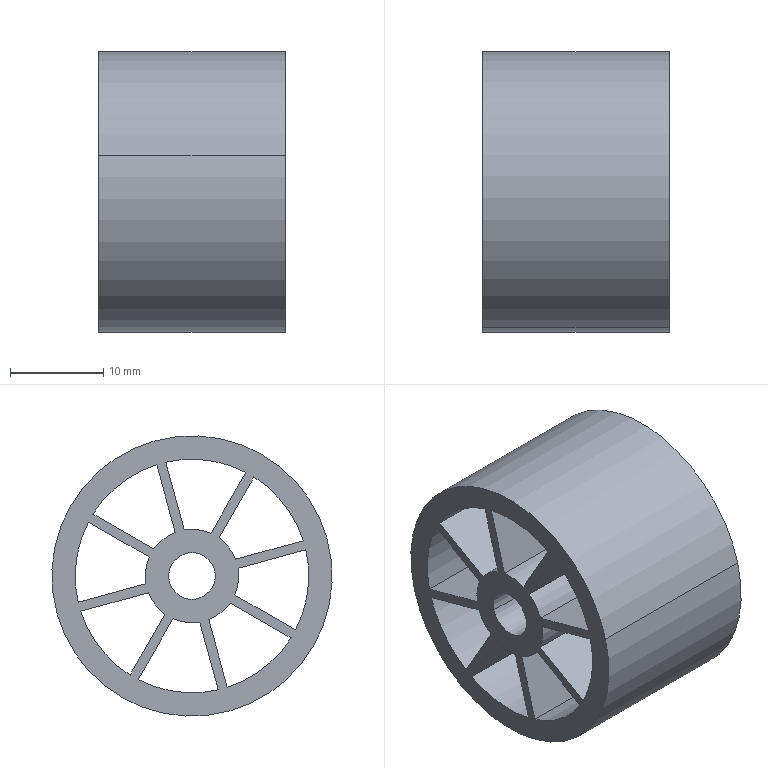Part | STEP file | Component42 | 1 solid | 38 faces | box 20 x 30 x 30 mm | volume 6699 mm3 | cylinder 20 | plane 18 | commonest cylinder face diameters 10 x8 25 x8 5 x2 30 x2
STEP:
#1=CARTESIAN_POINT('',(-10.,18.788,18.159));
#2=VERTEX_POINT('',#1);
#3=CARTESIAN_POINT('',(-10.,23.612,16.841));
#4=VERTEX_POINT('',#3);
#5=CARTESIAN_POINT('',(-10.,21.2,17.5));
#6=DIRECTION('',(1.,0.,0.));
#7=DIRECTION('',(0.,-0.9646,0.2636));
#8=AXIS2_PLACEMENT_3D('',#5,#6,#7);
#9=CIRCLE('',#8,2.5);
#10=EDGE_CURVE('',#2,#4,#9,.T.);
#11=ORIENTED_EDGE('',*,*,#10,.F.);
#12=CARTESIAN_POINT('',(10.,18.788,18.159));
#13=VERTEX_POINT('',#12);
#14=CARTESIAN_POINT('',(10.,18.788,18.159));
#15=DIRECTION('',(1.,0.,0.));
#16=VECTOR('',#15,1000.);
#17=LINE('',#14,#16);
#18=EDGE_CURVE('',#2,#13,#17,.T.);
#19=ORIENTED_EDGE('',*,*,#18,.T.);
#20=CARTESIAN_POINT('',(10.,23.612,16.841));
#21=VERTEX_POINT('',#20);
#22=CARTESIAN_POINT('',(10.,21.2,17.5));
#23=DIRECTION('',(1.,0.,0.));
#24=DIRECTION('',(0.,-0.9646,0.2636));
#25=AXIS2_PLACEMENT_3D('',#22,#23,#24);
#26=CIRCLE('',#25,2.5);
#27=EDGE_CURVE('',#13,#21,#26,.T.);
#28=ORIENTED_EDGE('',*,*,#27,.T.);
#29=CARTESIAN_POINT('',(10.,23.612,16.841));
#30=DIRECTION('',(1.,0.,0.));
#31=VECTOR('',#30,1000.);
#32=LINE('',#29,#31);
#33=EDGE_CURVE('',#4,#21,#32,.T.);
#34=ORIENTED_EDGE('',*,*,#33,.F.);
#35=EDGE_LOOP('',(#11,#19,#28,#34));
#36=FACE_OUTER_BOUND('',#35,.T.);
#37=CARTESIAN_POINT('',(10.,21.2,17.5));
#38=DIRECTION('',(1.,0.,0.));
#39=DIRECTION('',(0.,0.9646,-0.2636));
#40=AXIS2_PLACEMENT_3D('',#37,#38,#39);
#41=CYLINDRICAL_SURFACE('',#40,2.5);
#42=ADVANCED_FACE('',(#36),#41,.F.);
#43=CARTESIAN_POINT('',(-10.,35.67,13.547));
#44=VERTEX_POINT('',#43);
#45=CARTESIAN_POINT('',(-10.,6.73,21.453));
#46=VERTEX_POINT('',#45);
#47=CARTESIAN_POINT('',(-10.,21.2,17.5));
#48=DIRECTION('',(1.,0.,0.));
#49=DIRECTION('',(0.,-0.9646,0.2636));
#50=AXIS2_PLACEMENT_3D('',#47,#48,#49);
#51=CIRCLE('',#50,15.);
#52=EDGE_CURVE('',#44,#46,#51,.T.);
#53=ORIENTED_EDGE('',*,*,#52,.T.);
#54=CARTESIAN_POINT('',(10.,6.73,21.453));
#55=VERTEX_POINT('',#54);
#56=CARTESIAN_POINT('',(10.,6.73,21.453));
#57=DIRECTION('',(1.,0.,0.));
#58=VECTOR('',#57,1000.);
#59=LINE('',#56,#58);
#60=EDGE_CURVE('',#46,#55,#59,.T.);
#61=ORIENTED_EDGE('',*,*,#60,.T.);
#62=CARTESIAN_POINT('',(10.,35.67,13.547));
#63=VERTEX_POINT('',#62);
#64=CARTESIAN_POINT('',(10.,21.2,17.5));
#65=DIRECTION('',(1.,0.,0.));
#66=DIRECTION('',(0.,-0.9646,0.2636));
#67=AXIS2_PLACEMENT_3D('',#64,#65,#66);
#68=CIRCLE('',#67,15.);
#69=EDGE_CURVE('',#63,#55,#68,.T.);
#70=ORIENTED_EDGE('',*,*,#69,.F.);
#71=CARTESIAN_POINT('',(10.,35.67,13.547));
#72=DIRECTION('',(1.,0.,0.));
#73=VECTOR('',#72,1000.);
#74=LINE('',#71,#73);
#75=EDGE_CURVE('',#44,#63,#74,.T.);
#76=ORIENTED_EDGE('',*,*,#75,.F.);
#77=EDGE_LOOP('',(#53,#61,#70,#76));
#78=FACE_OUTER_BOUND('',#77,.T.);
#79=CARTESIAN_POINT('',(10.,21.2,17.5));
#80=DIRECTION('',(1.,0.,0.));
#81=DIRECTION('',(0.,0.9646,-0.2636));
#82=AXIS2_PLACEMENT_3D('',#79,#80,#81);
#83=CYLINDRICAL_SURFACE('',#82,15.);
#84=ADVANCED_FACE('',(#78),#83,.T.);
#85=CARTESIAN_POINT('',(10.,33.117,13.726));
#86=VERTEX_POINT('',#85);
#87=CARTESIAN_POINT('',(10.,25.867,15.706));
#88=VERTEX_POINT('',#87);
#89=CARTESIAN_POINT('',(10.,33.117,13.726));
#90=DIRECTION('',(0.,-0.9646,0.2636));
#91=VECTOR('',#90,1000.);
#92=LINE('',#89,#91);
#93=EDGE_CURVE('',#86,#88,#92,.T.);
#94=ORIENTED_EDGE('',*,*,#93,.T.);
#95=CARTESIAN_POINT('',(-10.,25.867,15.706));
#96=VERTEX_POINT('',#95);
#97=CARTESIAN_POINT('',(-10.,25.867,15.706));
#98=DIRECTION('',(1.,0.,0.));
#99=VECTOR('',#98,1000.);
#100=LINE('',#97,#99);
#101=EDGE_CURVE('',#96,#88,#100,.T.);
#102=ORIENTED_EDGE('',*,*,#101,.F.);
#103=CARTESIAN_POINT('',(-10.,33.117,13.726));
#104=VERTEX_POINT('',#103);
#105=CARTESIAN_POINT('',(-10.,33.117,13.726));
#106=DIRECTION('',(0.,-0.9646,0.2636));
#107=VECTOR('',#106,1000.);
#108=LINE('',#105,#107);
#109=EDGE_CURVE('',#104,#96,#108,.T.);
#110=ORIENTED_EDGE('',*,*,#109,.F.);
#111=CARTESIAN_POINT('',(-10.,33.117,13.726));
#112=DIRECTION('',(1.,0.,0.));
#113=VECTOR('',#112,1000.);
#114=LINE('',#111,#113);
#115=EDGE_CURVE('',#104,#86,#114,.T.);
#116=ORIENTED_EDGE('',*,*,#115,.T.);
#117=EDGE_LOOP('',(#94,#102,#110,#116));
#118=FACE_OUTER_BOUND('',#117,.T.);
#119=CARTESIAN_POINT('',(-10.,29.492,14.716));
#120=DIRECTION('',(0.,0.2636,0.9646));
#121=DIRECTION('',(1.,0.,0.));
#122=AXIS2_PLACEMENT_3D('',#119,#120,#121);
#123=PLANE('',#122);
#124=ADVANCED_FACE('',(#118),#123,.F.);
#125=CARTESIAN_POINT('',(10.,27.826,6.901));
#126=VERTEX_POINT('',#125);
#127=CARTESIAN_POINT('',(10.,21.2,17.5));
#128=DIRECTION('',(1.,0.,0.));
#129=DIRECTION('',(0.,-0.9646,0.2636));
#130=AXIS2_PLACEMENT_3D('',#127,#128,#129);
#131=CIRCLE('',#130,12.5);
#132=EDGE_CURVE('',#126,#86,#131,.T.);
#133=ORIENTED_EDGE('',*,*,#132,.T.);
#134=ORIENTED_EDGE('',*,*,#115,.F.);
#135=CARTESIAN_POINT('',(-10.,27.826,6.901));
#136=VERTEX_POINT('',#135);
#137=CARTESIAN_POINT('',(-10.,21.2,17.5));
#138=DIRECTION('',(1.,0.,0.));
#139=DIRECTION('',(0.,-0.9646,0.2636));
#140=AXIS2_PLACEMENT_3D('',#137,#138,#139);
#141=CIRCLE('',#140,12.5);
#142=EDGE_CURVE('',#136,#104,#141,.T.);
#143=ORIENTED_EDGE('',*,*,#142,.F.);
#144=CARTESIAN_POINT('',(-10.,27.826,6.901));
#145=DIRECTION('',(1.,0.,0.));
#146=VECTOR('',#145,1000.);
#147=LINE('',#144,#146);
#148=EDGE_CURVE('',#136,#126,#147,.T.);
#149=ORIENTED_EDGE('',*,*,#148,.T.);
#150=EDGE_LOOP('',(#133,#134,#143,#149));
#151=FACE_OUTER_BOUND('',#150,.T.);
#152=CARTESIAN_POINT('',(-10.,21.2,17.5));
#153=DIRECTION('',(-1.,0.,0.));
#154=DIRECTION('',(0.,-0.9646,0.2636));
#155=AXIS2_PLACEMENT_3D('',#152,#153,#154);
#156=CYLINDRICAL_SURFACE('',#155,12.5);
#157=ADVANCED_FACE('',(#151),#156,.F.);
#158=CARTESIAN_POINT('',(10.,24.101,13.427));
#159=VERTEX_POINT('',#158);
#160=CARTESIAN_POINT('',(10.,24.101,13.427));
#161=DIRECTION('',(0.,0.4957,-0.8685));
#162=VECTOR('',#161,1000.);
#163=LINE('',#160,#162);
#164=EDGE_CURVE('',#159,#126,#163,.T.);
#165=ORIENTED_EDGE('',*,*,#164,.T.);
#166=ORIENTED_EDGE('',*,*,#148,.F.);
#167=CARTESIAN_POINT('',(-10.,24.101,13.427));
#168=VERTEX_POINT('',#167);
#169=CARTESIAN_POINT('',(-10.,24.101,13.427));
#170=DIRECTION('',(0.,0.4957,-0.8685));
#171=VECTOR('',#170,1000.);
#172=LINE('',#169,#171);
#173=EDGE_CURVE('',#168,#136,#172,.T.);
#174=ORIENTED_EDGE('',*,*,#173,.F.);
#175=CARTESIAN_POINT('',(-10.,24.101,13.427));
#176=DIRECTION('',(1.,0.,0.));
#177=VECTOR('',#176,1000.);
#178=LINE('',#175,#177);
#179=EDGE_CURVE('',#168,#159,#178,.T.);
#180=ORIENTED_EDGE('',*,*,#179,.T.);
#181=EDGE_LOOP('',(#165,#166,#174,#180));
#182=FACE_OUTER_BOUND('',#181,.T.);
#183=CARTESIAN_POINT('',(-10.,25.963,10.164));
#184=DIRECTION('',(0.,-0.8685,-0.4957));
#185=DIRECTION('',(0.,0.4957,-0.8685));
#186=AXIS2_PLACEMENT_3D('',#183,#184,#185);
#187=PLANE('',#186);
#188=ADVANCED_FACE('',(#182),#187,.F.);
#189=CARTESIAN_POINT('',(10.,21.2,17.5));
#190=DIRECTION('',(-1.,0.,0.));
#191=DIRECTION('',(0.,-0.9646,0.2636));
#192=AXIS2_PLACEMENT_3D('',#189,#190,#191);
#193=CIRCLE('',#192,5.);
#194=EDGE_CURVE('',#88,#159,#193,.T.);
#195=ORIENTED_EDGE('',*,*,#194,.T.);
#196=ORIENTED_EDGE('',*,*,#179,.F.);
#197=CARTESIAN_POINT('',(-10.,21.2,17.5));
#198=DIRECTION('',(-1.,0.,0.));
#199=DIRECTION('',(0.,-0.9646,0.2636));
#200=AXIS2_PLACEMENT_3D('',#197,#198,#199);
#201=CIRCLE('',#200,5.);
#202=EDGE_CURVE('',#96,#168,#201,.T.);
#203=ORIENTED_EDGE('',*,*,#202,.F.);
#204=ORIENTED_EDGE('',*,*,#101,.T.);
#205=EDGE_LOOP('',(#195,#196,#203,#204));
#206=FACE_OUTER_BOUND('',#205,.T.);
#207=CARTESIAN_POINT('',(-10.,21.2,17.5));
#208=DIRECTION('',(-1.,0.,0.));
#209=DIRECTION('',(0.,-0.9646,0.2636));
#210=AXIS2_PLACEMENT_3D('',#207,#208,#209);
#211=CYLINDRICAL_SURFACE('',#210,5.);
#212=ADVANCED_FACE('',(#206),#211,.T.);
#213=CARTESIAN_POINT('',(10.,32.295,23.258));
#214=VERTEX_POINT('',#213);
#215=CARTESIAN_POINT('',(10.,25.768,19.532));
#216=VERTEX_POINT('',#215);
#217=CARTESIAN_POINT('',(10.,32.295,23.258));
#218=DIRECTION('',(0.,-0.8685,-0.4957));
#219=VECTOR('',#218,1000.);
#220=LINE('',#217,#219);
#221=EDGE_CURVE('',#214,#216,#220,.T.);
#222=ORIENTED_EDGE('',*,*,#221,.T.);
#223=CARTESIAN_POINT('',(-10.,25.768,19.532));
#224=VERTEX_POINT('',#223);
#225=CARTESIAN_POINT('',(-10.,25.768,19.532));
#226=DIRECTION('',(1.,0.,0.));
#227=VECTOR('',#226,1000.);
#228=LINE('',#225,#227);
#229=EDGE_CURVE('',#224,#216,#228,.T.);
#230=ORIENTED_EDGE('',*,*,#229,.F.);
#231=CARTESIAN_POINT('',(-10.,32.295,23.258));
#232=VERTEX_POINT('',#231);
#233=CARTESIAN_POINT('',(-10.,32.295,23.258));
#234=DIRECTION('',(0.,-0.8685,-0.4957));
#235=VECTOR('',#234,1000.);
#236=LINE('',#233,#235);
#237=EDGE_CURVE('',#232,#224,#236,.T.);
#238=ORIENTED_EDGE('',*,*,#237,.F.);
#239=CARTESIAN_POINT('',(-10.,32.295,23.258));
#240=DIRECTION('',(1.,0.,0.));
#241=VECTOR('',#240,1000.);
#242=LINE('',#239,#241);
#243=EDGE_CURVE('',#232,#214,#242,.T.);
#244=ORIENTED_EDGE('',*,*,#243,.T.);
#245=EDGE_LOOP('',(#222,#230,#238,#244));
#246=FACE_OUTER_BOUND('',#245,.T.);
#247=CARTESIAN_POINT('',(-10.,29.032,21.395));
#248=DIRECTION('',(0.,-0.4957,0.8685));
#249=DIRECTION('',(-1.,0.,0.));
#250=AXIS2_PLACEMENT_3D('',#247,#248,#249);
#251=PLANE('',#250);
#252=ADVANCED_FACE('',(#246),#251,.F.);
#253=CARTESIAN_POINT('',(10.,33.38,14.69));
#254=VERTEX_POINT('',#253);
#255=CARTESIAN_POINT('',(10.,21.2,17.5));
#256=DIRECTION('',(1.,0.,0.));
#257=DIRECTION('',(0.,-0.9646,0.2636));
#258=AXIS2_PLACEMENT_3D('',#255,#256,#257);
#259=CIRCLE('',#258,12.5);
#260=EDGE_CURVE('',#254,#214,#259,.T.);
#261=ORIENTED_EDGE('',*,*,#260,.T.);
#262=ORIENTED_EDGE('',*,*,#243,.F.);
#263=CARTESIAN_POINT('',(-10.,33.38,14.69));
#264=VERTEX_POINT('',#263);
#265=CARTESIAN_POINT('',(-10.,21.2,17.5));
#266=DIRECTION('',(1.,0.,0.));
#267=DIRECTION('',(0.,-0.9646,0.2636));
#268=AXIS2_PLACEMENT_3D('',#265,#266,#267);
#269=CIRCLE('',#268,12.5);
#270=EDGE_CURVE('',#264,#232,#269,.T.);
#271=ORIENTED_EDGE('',*,*,#270,.F.);
#272=CARTESIAN_POINT('',(-10.,33.38,14.69));
#273=DIRECTION('',(1.,0.,0.));
#274=VECTOR('',#273,1000.);
#275=LINE('',#272,#274);
#276=EDGE_CURVE('',#264,#254,#275,.T.);
#277=ORIENTED_EDGE('',*,*,#276,.T.);
#278=EDGE_LOOP('',(#261,#262,#271,#277));
#279=FACE_OUTER_BOUND('',#278,.T.);
#280=CARTESIAN_POINT('',(-10.,21.2,17.5));
#281=DIRECTION('',(-1.,0.,0.));
#282=DIRECTION('',(0.,-0.9646,0.2636));
#283=AXIS2_PLACEMENT_3D('',#280,#281,#282);
#284=CYLINDRICAL_SURFACE('',#283,12.5);
#285=ADVANCED_FACE('',(#279),#284,.F.);
#286=CARTESIAN_POINT('',(10.,26.131,16.671));
#287=VERTEX_POINT('',#286);
#288=CARTESIAN_POINT('',(10.,26.131,16.671));
#289=DIRECTION('',(0.,0.9646,-0.2636));
#290=VECTOR('',#289,1000.);
#291=LINE('',#288,#290);
#292=EDGE_CURVE('',#287,#254,#291,.T.);
#293=ORIENTED_EDGE('',*,*,#292,.T.);
#294=ORIENTED_EDGE('',*,*,#276,.F.);
#295=CARTESIAN_POINT('',(-10.,26.131,16.671));
#296=VERTEX_POINT('',#295);
#297=CARTESIAN_POINT('',(-10.,26.131,16.671));
#298=DIRECTION('',(0.,0.9646,-0.2636));
#299=VECTOR('',#298,1000.);
#300=LINE('',#297,#299);
#301=EDGE_CURVE('',#296,#264,#300,.T.);
#302=ORIENTED_EDGE('',*,*,#301,.F.);
#303=CARTESIAN_POINT('',(-10.,26.131,16.671));
#304=DIRECTION('',(1.,0.,0.));
#305=VECTOR('',#304,1000.);
#306=LINE('',#303,#305);
#307=EDGE_CURVE('',#296,#287,#306,.T.);
#308=ORIENTED_EDGE('',*,*,#307,.T.);
#309=EDGE_LOOP('',(#293,#294,#302,#308));
#310=FACE_OUTER_BOUND('',#309,.T.);
#311=CARTESIAN_POINT('',(-10.,29.755,15.681));
#312=DIRECTION('',(0.,-0.2636,-0.9646));
#313=DIRECTION('',(0.,-0.9646,0.2636));
#314=AXIS2_PLACEMENT_3D('',#311,#312,#313);
#315=PLANE('',#314);
#316=ADVANCED_FACE('',(#310),#315,.F.);
#317=CARTESIAN_POINT('',(10.,21.2,17.5));
#318=DIRECTION('',(-1.,0.,0.));
#319=DIRECTION('',(0.,-0.9646,0.2636));
#320=AXIS2_PLACEMENT_3D('',#317,#318,#319);
#321=CIRCLE('',#320,5.);
#322=EDGE_CURVE('',#216,#287,#321,.T.);
#323=ORIENTED_EDGE('',*,*,#322,.T.);
#324=ORIENTED_EDGE('',*,*,#307,.F.);
#325=CARTESIAN_POINT('',(-10.,21.2,17.5));
#326=DIRECTION('',(-1.,0.,0.));
#327=DIRECTION('',(0.,-0.9646,0.2636));
#328=AXIS2_PLACEMENT_3D('',#325,#326,#327);
#329=CIRCLE('',#328,5.);
#330=EDGE_CURVE('',#224,#296,#329,.T.);
#331=ORIENTED_EDGE('',*,*,#330,.F.);
#332=ORIENTED_EDGE('',*,*,#229,.T.);
#333=EDGE_LOOP('',(#323,#324,#331,#332));
#334=FACE_OUTER_BOUND('',#333,.T.);
#335=CARTESIAN_POINT('',(-10.,21.2,17.5));
#336=DIRECTION('',(-1.,0.,0.));
#337=DIRECTION('',(0.,-0.9646,0.2636));
#338=AXIS2_PLACEMENT_3D('',#335,#336,#337);
#339=CYLINDRICAL_SURFACE('',#338,5.);
#340=ADVANCED_FACE('',(#334),#339,.T.);
#341=CARTESIAN_POINT('',(10.,24.974,29.417));
#342=VERTEX_POINT('',#341);
#343=CARTESIAN_POINT('',(10.,22.994,22.167));
#344=VERTEX_POINT('',#343);
#345=CARTESIAN_POINT('',(10.,24.974,29.417));
#346=DIRECTION('',(0.,-0.2636,-0.9646));
#347=VECTOR('',#346,1000.);
#348=LINE('',#345,#347);
#349=EDGE_CURVE('',#342,#344,#348,.T.);
#350=ORIENTED_EDGE('',*,*,#349,.T.);
#351=CARTESIAN_POINT('',(-10.,22.994,22.167));
#352=VERTEX_POINT('',#351);
#353=CARTESIAN_POINT('',(-10.,22.994,22.167));
#354=DIRECTION('',(1.,0.,0.));
#355=VECTOR('',#354,1000.);
#356=LINE('',#353,#355);
#357=EDGE_CURVE('',#352,#344,#356,.T.);
#358=ORIENTED_EDGE('',*,*,#357,.F.);
#359=CARTESIAN_POINT('',(-10.,24.974,29.417));
#360=VERTEX_POINT('',#359);
#361=CARTESIAN_POINT('',(-10.,24.974,29.417));
#362=DIRECTION('',(0.,-0.2636,-0.9646));
#363=VECTOR('',#362,1000.);
#364=LINE('',#361,#363);
#365=EDGE_CURVE('',#360,#352,#364,.T.);
#366=ORIENTED_EDGE('',*,*,#365,.F.);
#367=CARTESIAN_POINT('',(-10.,24.974,29.417));
#368=DIRECTION('',(1.,0.,0.));
#369=VECTOR('',#368,1000.);
#370=LINE('',#367,#369);
#371=EDGE_CURVE('',#360,#342,#370,.T.);
#372=ORIENTED_EDGE('',*,*,#371,.T.);
#373=EDGE_LOOP('',(#350,#358,#366,#372));
#374=FACE_OUTER_BOUND('',#373,.T.);
#375=CARTESIAN_POINT('',(-10.,23.984,25.792));
#376=DIRECTION('',(0.,-0.9646,0.2636));
#377=DIRECTION('',(-1.,0.,0.));
#378=AXIS2_PLACEMENT_3D('',#375,#376,#377);
#379=PLANE('',#378);
#380=ADVANCED_FACE('',(#374),#379,.F.);
#381=CARTESIAN_POINT('',(10.,31.799,24.126));
#382=VERTEX_POINT('',#381);
#383=CARTESIAN_POINT('',(10.,21.2,17.5));
#384=DIRECTION('',(1.,0.,0.));
#385=DIRECTION('',(0.,-0.9646,0.2636));
#386=AXIS2_PLACEMENT_3D('',#383,#384,#385);
#387=CIRCLE('',#386,12.5);
#388=EDGE_CURVE('',#382,#342,#387,.T.);
#389=ORIENTED_EDGE('',*,*,#388,.T.);
#390=ORIENTED_EDGE('',*,*,#371,.F.);
#391=CARTESIAN_POINT('',(-10.,31.799,24.126));
#392=VERTEX_POINT('',#391);
#393=CARTESIAN_POINT('',(-10.,21.2,17.5));
#394=DIRECTION('',(1.,0.,0.));
#395=DIRECTION('',(0.,-0.9646,0.2636));
#396=AXIS2_PLACEMENT_3D('',#393,#394,#395);
#397=CIRCLE('',#396,12.5);
#398=EDGE_CURVE('',#392,#360,#397,.T.);
#399=ORIENTED_EDGE('',*,*,#398,.F.);
#400=CARTESIAN_POINT('',(-10.,31.799,24.126));
#401=DIRECTION('',(1.,0.,0.));
#402=VECTOR('',#401,1000.);
#403=LINE('',#400,#402);
#404=EDGE_CURVE('',#392,#382,#403,.T.);
#405=ORIENTED_EDGE('',*,*,#404,.T.);
#406=EDGE_LOOP('',(#389,#390,#399,#405));
#407=FACE_OUTER_BOUND('',#406,.T.);
#408=CARTESIAN_POINT('',(-10.,21.2,17.5));
#409=DIRECTION('',(-1.,0.,0.));
#410=DIRECTION('',(0.,-0.9646,0.2636));
#411=AXIS2_PLACEMENT_3D('',#408,#409,#410);
#412=CYLINDRICAL_SURFACE('',#411,12.5);
#413=ADVANCED_FACE('',(#407),#412,.F.);
#414=CARTESIAN_POINT('',(10.,25.273,20.401));
#415=VERTEX_POINT('',#414);
#416=CARTESIAN_POINT('',(10.,25.273,20.401));
#417=DIRECTION('',(0.,0.8685,0.4957));
#418=VECTOR('',#417,1000.);
#419=LINE('',#416,#418);
#420=EDGE_CURVE('',#415,#382,#419,.T.);
#421=ORIENTED_EDGE('',*,*,#420,.T.);
#422=ORIENTED_EDGE('',*,*,#404,.F.);
#423=CARTESIAN_POINT('',(-10.,25.273,20.401));
#424=VERTEX_POINT('',#423);
#425=CARTESIAN_POINT('',(-10.,25.273,20.401));
#426=DIRECTION('',(0.,0.8685,0.4957));
#427=VECTOR('',#426,1000.);
#428=LINE('',#425,#427);
#429=EDGE_CURVE('',#424,#392,#428,.T.);
#430=ORIENTED_EDGE('',*,*,#429,.F.);
#431=CARTESIAN_POINT('',(-10.,25.273,20.401));
#432=DIRECTION('',(1.,0.,0.));
#433=VECTOR('',#432,1000.);
#434=LINE('',#431,#433);
#435=EDGE_CURVE('',#424,#415,#434,.T.);
#436=ORIENTED_EDGE('',*,*,#435,.T.);
#437=EDGE_LOOP('',(#421,#422,#430,#436));
#438=FACE_OUTER_BOUND('',#437,.T.);
#439=CARTESIAN_POINT('',(-10.,28.536,22.263));
#440=DIRECTION('',(0.,0.4957,-0.8685));
#441=DIRECTION('',(-1.,0.,0.));
#442=AXIS2_PLACEMENT_3D('',#439,#440,#441);
#443=PLANE('',#442);
#444=ADVANCED_FACE('',(#438),#443,.F.);
#445=CARTESIAN_POINT('',(10.,21.2,17.5));
#446=DIRECTION('',(-1.,0.,0.));
#447=DIRECTION('',(0.,-0.9646,0.2636));
#448=AXIS2_PLACEMENT_3D('',#445,#446,#447);
#449=CIRCLE('',#448,5.);
#450=EDGE_CURVE('',#344,#415,#449,.T.);
#451=ORIENTED_EDGE('',*,*,#450,.T.);
#452=ORIENTED_EDGE('',*,*,#435,.F.);
#453=CARTESIAN_POINT('',(-10.,21.2,17.5));
#454=DIRECTION('',(-1.,0.,0.));
#455=DIRECTION('',(0.,-0.9646,0.2636));
#456=AXIS2_PLACEMENT_3D('',#453,#454,#455);
#457=CIRCLE('',#456,5.);
#458=EDGE_CURVE('',#352,#424,#457,.T.);
#459=ORIENTED_EDGE('',*,*,#458,.F.);
#460=ORIENTED_EDGE('',*,*,#357,.T.);
#461=EDGE_LOOP('',(#451,#452,#459,#460));
#462=FACE_OUTER_BOUND('',#461,.T.);
#463=CARTESIAN_POINT('',(-10.,21.2,17.5));
#464=DIRECTION('',(-1.,0.,0.));
#465=DIRECTION('',(0.,-0.9646,0.2636));
#466=AXIS2_PLACEMENT_3D('',#463,#464,#465);
#467=CYLINDRICAL_SURFACE('',#466,5.);
#468=ADVANCED_FACE('',(#462),#467,.T.);
#469=CARTESIAN_POINT('',(10.,15.442,28.595));
#470=VERTEX_POINT('',#469);
#471=CARTESIAN_POINT('',(10.,19.168,22.068));
#472=VERTEX_POINT('',#471);
#473=CARTESIAN_POINT('',(10.,15.442,28.595));
#474=DIRECTION('',(0.,0.4957,-0.8685));
#475=VECTOR('',#474,1000.);
#476=LINE('',#473,#475);
#477=EDGE_CURVE('',#470,#472,#476,.T.);
#478=ORIENTED_EDGE('',*,*,#477,.T.);
#479=CARTESIAN_POINT('',(-10.,19.168,22.068));
#480=VERTEX_POINT('',#479);
#481=CARTESIAN_POINT('',(-10.,19.168,22.068));
#482=DIRECTION('',(1.,0.,0.));
#483=VECTOR('',#482,1000.);
#484=LINE('',#481,#483);
#485=EDGE_CURVE('',#480,#472,#484,.T.);
#486=ORIENTED_EDGE('',*,*,#485,.F.);
#487=CARTESIAN_POINT('',(-10.,15.442,28.595));
#488=VERTEX_POINT('',#487);
#489=CARTESIAN_POINT('',(-10.,15.442,28.595));
#490=DIRECTION('',(0.,0.4957,-0.8685));
#491=VECTOR('',#490,1000.);
#492=LINE('',#489,#491);
#493=EDGE_CURVE('',#488,#480,#492,.T.);
#494=ORIENTED_EDGE('',*,*,#493,.F.);
#495=CARTESIAN_POINT('',(-10.,15.442,28.595));
#496=DIRECTION('',(1.,0.,0.));
#497=VECTOR('',#496,1000.);
#498=LINE('',#495,#497);
#499=EDGE_CURVE('',#488,#470,#498,.T.);
#500=ORIENTED_EDGE('',*,*,#499,.T.);
#501=EDGE_LOOP('',(#478,#486,#494,#500));
#502=FACE_OUTER_BOUND('',#501,.T.);
#503=CARTESIAN_POINT('',(-10.,17.305,25.332));
#504=DIRECTION('',(0.,-0.8685,-0.4957));
#505=DIRECTION('',(0.,0.4957,-0.8685));
#506=AXIS2_PLACEMENT_3D('',#503,#504,#505);
#507=PLANE('',#506);
#508=ADVANCED_FACE('',(#502),#507,.F.);
#509=CARTESIAN_POINT('',(10.,24.01,29.68));
#510=VERTEX_POINT('',#509);
#511=CARTESIAN_POINT('',(10.,21.2,17.5));
#512=DIRECTION('',(1.,0.,0.));
#513=DIRECTION('',(0.,-0.9646,0.2636));
#514=AXIS2_PLACEMENT_3D('',#511,#512,#513);
#515=CIRCLE('',#514,12.5);
#516=EDGE_CURVE('',#510,#470,#515,.T.);
#517=ORIENTED_EDGE('',*,*,#516,.T.);
#518=ORIENTED_EDGE('',*,*,#499,.F.);
#519=CARTESIAN_POINT('',(-10.,24.01,29.68));
#520=VERTEX_POINT('',#519);
#521=CARTESIAN_POINT('',(-10.,21.2,17.5));
#522=DIRECTION('',(1.,0.,0.));
#523=DIRECTION('',(0.,-0.9646,0.2636));
#524=AXIS2_PLACEMENT_3D('',#521,#522,#523);
#525=CIRCLE('',#524,12.5);
#526=EDGE_CURVE('',#520,#488,#525,.T.);
#527=ORIENTED_EDGE('',*,*,#526,.F.);
#528=CARTESIAN_POINT('',(-10.,24.01,29.68));
#529=DIRECTION('',(1.,0.,0.));
#530=VECTOR('',#529,1000.);
#531=LINE('',#528,#530);
#532=EDGE_CURVE('',#520,#510,#531,.T.);
#533=ORIENTED_EDGE('',*,*,#532,.T.);
#534=EDGE_LOOP('',(#517,#518,#527,#533));
#535=FACE_OUTER_BOUND('',#534,.T.);
#536=CARTESIAN_POINT('',(-10.,21.2,17.5));
#537=DIRECTION('',(-1.,0.,0.));
#538=DIRECTION('',(0.,-0.9646,0.2636));
#539=AXIS2_PLACEMENT_3D('',#536,#537,#538);
#540=CYLINDRICAL_SURFACE('',#539,12.5);
#541=ADVANCED_FACE('',(#535),#540,.F.);
#542=CARTESIAN_POINT('',(10.,22.029,22.431));
#543=VERTEX_POINT('',#542);
#544=CARTESIAN_POINT('',(10.,22.029,22.431));
#545=DIRECTION('',(0.,0.2636,0.9646));
#546=VECTOR('',#545,1000.);
#547=LINE('',#544,#546);
#548=EDGE_CURVE('',#543,#510,#547,.T.);
#549=ORIENTED_EDGE('',*,*,#548,.T.);
#550=ORIENTED_EDGE('',*,*,#532,.F.);
#551=CARTESIAN_POINT('',(-10.,22.029,22.431));
#552=VERTEX_POINT('',#551);
#553=CARTESIAN_POINT('',(-10.,22.029,22.431));
#554=DIRECTION('',(0.,0.2636,0.9646));
#555=VECTOR('',#554,1000.);
#556=LINE('',#553,#555);
#557=EDGE_CURVE('',#552,#520,#556,.T.);
#558=ORIENTED_EDGE('',*,*,#557,.F.);
#559=CARTESIAN_POINT('',(-10.,22.029,22.431));
#560=DIRECTION('',(1.,0.,0.));
#561=VECTOR('',#560,1000.);
#562=LINE('',#559,#561);
#563=EDGE_CURVE('',#552,#543,#562,.T.);
#564=ORIENTED_EDGE('',*,*,#563,.T.);
#565=EDGE_LOOP('',(#549,#550,#558,#564));
#566=FACE_OUTER_BOUND('',#565,.T.);
#567=CARTESIAN_POINT('',(-10.,23.019,26.055));
#568=DIRECTION('',(0.,0.9646,-0.2636));
#569=DIRECTION('',(-1.,0.,0.));
#570=AXIS2_PLACEMENT_3D('',#567,#568,#569);
#571=PLANE('',#570);
#572=ADVANCED_FACE('',(#566),#571,.F.);
#573=CARTESIAN_POINT('',(10.,21.2,17.5));
#574=DIRECTION('',(-1.,0.,0.));
#575=DIRECTION('',(0.,-0.9646,0.2636));
#576=AXIS2_PLACEMENT_3D('',#573,#574,#575);
#577=CIRCLE('',#576,5.);
#578=EDGE_CURVE('',#472,#543,#577,.T.);
#579=ORIENTED_EDGE('',*,*,#578,.T.);
#580=ORIENTED_EDGE('',*,*,#563,.F.);
#581=CARTESIAN_POINT('',(-10.,21.2,17.5));
#582=DIRECTION('',(-1.,0.,0.));
#583=DIRECTION('',(0.,-0.9646,0.2636));
#584=AXIS2_PLACEMENT_3D('',#581,#582,#583);
#585=CIRCLE('',#584,5.);
#586=EDGE_CURVE('',#480,#552,#585,.T.);
#587=ORIENTED_EDGE('',*,*,#586,.F.);
#588=ORIENTED_EDGE('',*,*,#485,.T.);
#589=EDGE_LOOP('',(#579,#580,#587,#588));
#590=FACE_OUTER_BOUND('',#589,.T.);
#591=CARTESIAN_POINT('',(-10.,21.2,17.5));
#592=DIRECTION('',(-1.,0.,0.));
#593=DIRECTION('',(0.,-0.9646,0.2636));
#594=AXIS2_PLACEMENT_3D('',#591,#592,#593);
#595=CYLINDRICAL_SURFACE('',#594,5.);
#596=ADVANCED_FACE('',(#590),#595,.T.);
#597=CARTESIAN_POINT('',(10.,9.283,21.274));
#598=VERTEX_POINT('',#597);
#599=CARTESIAN_POINT('',(10.,16.533,19.294));
#600=VERTEX_POINT('',#599);
#601=CARTESIAN_POINT('',(10.,9.283,21.274));
#602=DIRECTION('',(0.,0.9646,-0.2636));
#603=VECTOR('',#602,1000.);
#604=LINE('',#601,#603);
#605=EDGE_CURVE('',#598,#600,#604,.T.);
#606=ORIENTED_EDGE('',*,*,#605,.T.);
#607=CARTESIAN_POINT('',(-10.,16.533,19.294));
#608=VERTEX_POINT('',#607);
#609=CARTESIAN_POINT('',(-10.,16.533,19.294));
#610=DIRECTION('',(1.,0.,0.));
#611=VECTOR('',#610,1000.);
#612=LINE('',#609,#611);
#613=EDGE_CURVE('',#608,#600,#612,.T.);
#614=ORIENTED_EDGE('',*,*,#613,.F.);
#615=CARTESIAN_POINT('',(-10.,9.283,21.274));
#616=VERTEX_POINT('',#615);
#617=CARTESIAN_POINT('',(-10.,9.283,21.274));
#618=DIRECTION('',(0.,0.9646,-0.2636));
#619=VECTOR('',#618,1000.);
#620=LINE('',#617,#619);
#621=EDGE_CURVE('',#616,#608,#620,.T.);
#622=ORIENTED_EDGE('',*,*,#621,.F.);
#623=CARTESIAN_POINT('',(-10.,9.283,21.274));
#624=DIRECTION('',(1.,0.,0.));
#625=VECTOR('',#624,1000.);
#626=LINE('',#623,#625);
#627=EDGE_CURVE('',#616,#598,#626,.T.);
#628=ORIENTED_EDGE('',*,*,#627,.T.);
#629=EDGE_LOOP('',(#606,#614,#622,#628));
#630=FACE_OUTER_BOUND('',#629,.T.);
#631=CARTESIAN_POINT('',(-10.,12.908,20.284));
#632=DIRECTION('',(0.,-0.2636,-0.9646));
#633=DIRECTION('',(0.,-0.9646,0.2636));
#634=AXIS2_PLACEMENT_3D('',#631,#632,#633);
#635=PLANE('',#634);
#636=ADVANCED_FACE('',(#630),#635,.F.);
#637=CARTESIAN_POINT('',(10.,14.574,28.099));
#638=VERTEX_POINT('',#637);
#639=CARTESIAN_POINT('',(10.,21.2,17.5));
#640=DIRECTION('',(1.,0.,0.));
#641=DIRECTION('',(0.,-0.9646,0.2636));
#642=AXIS2_PLACEMENT_3D('',#639,#640,#641);
#643=CIRCLE('',#642,12.5);
#644=EDGE_CURVE('',#638,#598,#643,.T.);
#645=ORIENTED_EDGE('',*,*,#644,.T.);
#646=ORIENTED_EDGE('',*,*,#627,.F.);
#647=CARTESIAN_POINT('',(-10.,14.574,28.099));
#648=VERTEX_POINT('',#647);
#649=CARTESIAN_POINT('',(-10.,21.2,17.5));
#650=DIRECTION('',(1.,0.,0.));
#651=DIRECTION('',(0.,-0.9646,0.2636));
#652=AXIS2_PLACEMENT_3D('',#649,#650,#651);
#653=CIRCLE('',#652,12.5);
#654=EDGE_CURVE('',#648,#616,#653,.T.);
#655=ORIENTED_EDGE('',*,*,#654,.F.);
#656=CARTESIAN_POINT('',(-10.,14.574,28.099));
#657=DIRECTION('',(1.,0.,0.));
#658=VECTOR('',#657,1000.);
#659=LINE('',#656,#658);
#660=EDGE_CURVE('',#648,#638,#659,.T.);
#661=ORIENTED_EDGE('',*,*,#660,.T.);
#662=EDGE_LOOP('',(#645,#646,#655,#661));
#663=FACE_OUTER_BOUND('',#662,.T.);
#664=CARTESIAN_POINT('',(-10.,21.2,17.5));
#665=DIRECTION('',(-1.,0.,0.));
#666=DIRECTION('',(0.,-0.9646,0.2636));
#667=AXIS2_PLACEMENT_3D('',#664,#665,#666);
#668=CYLINDRICAL_SURFACE('',#667,12.5);
#669=ADVANCED_FACE('',(#663),#668,.F.);
#670=CARTESIAN_POINT('',(10.,18.299,21.573));
#671=VERTEX_POINT('',#670);
#672=CARTESIAN_POINT('',(10.,18.299,21.573));
#673=DIRECTION('',(0.,-0.4957,0.8685));
#674=VECTOR('',#673,1000.);
#675=LINE('',#672,#674);
#676=EDGE_CURVE('',#671,#638,#675,.T.);
#677=ORIENTED_EDGE('',*,*,#676,.T.);
#678=ORIENTED_EDGE('',*,*,#660,.F.);
#679=CARTESIAN_POINT('',(-10.,18.299,21.573));
#680=VERTEX_POINT('',#679);
#681=CARTESIAN_POINT('',(-10.,18.299,21.573));
#682=DIRECTION('',(0.,-0.4957,0.8685));
#683=VECTOR('',#682,1000.);
#684=LINE('',#681,#683);
#685=EDGE_CURVE('',#680,#648,#684,.T.);
#686=ORIENTED_EDGE('',*,*,#685,.F.);
#687=CARTESIAN_POINT('',(-10.,18.299,21.573));
#688=DIRECTION('',(1.,0.,0.));
#689=VECTOR('',#688,1000.);
#690=LINE('',#687,#689);
#691=EDGE_CURVE('',#680,#671,#690,.T.);
#692=ORIENTED_EDGE('',*,*,#691,.T.);
#693=EDGE_LOOP('',(#677,#678,#686,#692));
#694=FACE_OUTER_BOUND('',#693,.T.);
#695=CARTESIAN_POINT('',(-10.,16.437,24.836));
#696=DIRECTION('',(0.,0.8685,0.4957));
#697=DIRECTION('',(1.,0.,0.));
#698=AXIS2_PLACEMENT_3D('',#695,#696,#697);
#699=PLANE('',#698);
#700=ADVANCED_FACE('',(#694),#699,.F.);
#701=CARTESIAN_POINT('',(10.,21.2,17.5));
#702=DIRECTION('',(-1.,0.,0.));
#703=DIRECTION('',(0.,-0.9646,0.2636));
#704=AXIS2_PLACEMENT_3D('',#701,#702,#703);
#705=CIRCLE('',#704,5.);
#706=EDGE_CURVE('',#600,#671,#705,.T.);
#707=ORIENTED_EDGE('',*,*,#706,.T.);
#708=ORIENTED_EDGE('',*,*,#691,.F.);
#709=CARTESIAN_POINT('',(-10.,21.2,17.5));
#710=DIRECTION('',(-1.,0.,0.));
#711=DIRECTION('',(0.,-0.9646,0.2636));
#712=AXIS2_PLACEMENT_3D('',#709,#710,#711);
#713=CIRCLE('',#712,5.);
#714=EDGE_CURVE('',#608,#680,#713,.T.);
#715=ORIENTED_EDGE('',*,*,#714,.F.);
#716=ORIENTED_EDGE('',*,*,#613,.T.);
#717=EDGE_LOOP('',(#707,#708,#715,#716));
#718=FACE_OUTER_BOUND('',#717,.T.);
#719=CARTESIAN_POINT('',(-10.,21.2,17.5));
#720=DIRECTION('',(-1.,0.,0.));
#721=DIRECTION('',(0.,-0.9646,0.2636));
#722=AXIS2_PLACEMENT_3D('',#719,#720,#721);
#723=CYLINDRICAL_SURFACE('',#722,5.);
#724=ADVANCED_FACE('',(#718),#723,.T.);
#725=CARTESIAN_POINT('',(10.,10.105,11.742));
#726=VERTEX_POINT('',#725);
#727=CARTESIAN_POINT('',(10.,16.632,15.468));
#728=VERTEX_POINT('',#727);
#729=CARTESIAN_POINT('',(10.,10.105,11.742));
#730=DIRECTION('',(0.,0.8685,0.4957));
#731=VECTOR('',#730,1000.);
#732=LINE('',#729,#731);
#733=EDGE_CURVE('',#726,#728,#732,.T.);
#734=ORIENTED_EDGE('',*,*,#733,.T.);
#735=CARTESIAN_POINT('',(-10.,16.632,15.468));
#736=VERTEX_POINT('',#735);
#737=CARTESIAN_POINT('',(-10.,16.632,15.468));
#738=DIRECTION('',(1.,0.,0.));
#739=VECTOR('',#738,1000.);
#740=LINE('',#737,#739);
#741=EDGE_CURVE('',#736,#728,#740,.T.);
#742=ORIENTED_EDGE('',*,*,#741,.F.);
#743=CARTESIAN_POINT('',(-10.,10.105,11.742));
#744=VERTEX_POINT('',#743);
#745=CARTESIAN_POINT('',(-10.,10.105,11.742));
#746=DIRECTION('',(0.,0.8685,0.4957));
#747=VECTOR('',#746,1000.);
#748=LINE('',#745,#747);
#749=EDGE_CURVE('',#744,#736,#748,.T.);
#750=ORIENTED_EDGE('',*,*,#749,.F.);
#751=CARTESIAN_POINT('',(-10.,10.105,11.742));
#752=DIRECTION('',(1.,0.,0.));
#753=VECTOR('',#752,1000.);
#754=LINE('',#751,#753);
#755=EDGE_CURVE('',#744,#726,#754,.T.);
#756=ORIENTED_EDGE('',*,*,#755,.T.);
#757=EDGE_LOOP('',(#734,#742,#750,#756));
#758=FACE_OUTER_BOUND('',#757,.T.);
#759=CARTESIAN_POINT('',(-10.,13.368,13.605));
#760=DIRECTION('',(0.,0.4957,-0.8685));
#761=DIRECTION('',(-1.,0.,0.));
#762=AXIS2_PLACEMENT_3D('',#759,#760,#761);
#763=PLANE('',#762);
#764=ADVANCED_FACE('',(#758),#763,.F.);
#765=CARTESIAN_POINT('',(10.,9.02,20.31));
#766=VERTEX_POINT('',#765);
#767=CARTESIAN_POINT('',(10.,21.2,17.5));
#768=DIRECTION('',(1.,0.,0.));
#769=DIRECTION('',(0.,-0.9646,0.2636));
#770=AXIS2_PLACEMENT_3D('',#767,#768,#769);
#771=CIRCLE('',#770,12.5);
#772=EDGE_CURVE('',#766,#726,#771,.T.);
#773=ORIENTED_EDGE('',*,*,#772,.T.);
#774=ORIENTED_EDGE('',*,*,#755,.F.);
#775=CARTESIAN_POINT('',(-10.,9.02,20.31));
#776=VERTEX_POINT('',#775);
#777=CARTESIAN_POINT('',(-10.,21.2,17.5));
#778=DIRECTION('',(1.,0.,0.));
#779=DIRECTION('',(0.,-0.9646,0.2636));
#780=AXIS2_PLACEMENT_3D('',#777,#778,#779);
#781=CIRCLE('',#780,12.5);
#782=EDGE_CURVE('',#776,#744,#781,.T.);
#783=ORIENTED_EDGE('',*,*,#782,.F.);
#784=CARTESIAN_POINT('',(-10.,9.02,20.31));
#785=DIRECTION('',(1.,0.,0.));
#786=VECTOR('',#785,1000.);
#787=LINE('',#784,#786);
#788=EDGE_CURVE('',#776,#766,#787,.T.);
#789=ORIENTED_EDGE('',*,*,#788,.T.);
#790=EDGE_LOOP('',(#773,#774,#783,#789));
#791=FACE_OUTER_BOUND('',#790,.T.);
#792=CARTESIAN_POINT('',(-10.,21.2,17.5));
#793=DIRECTION('',(-1.,0.,0.));
#794=DIRECTION('',(0.,-0.9646,0.2636));
#795=AXIS2_PLACEMENT_3D('',#792,#793,#794);
#796=CYLINDRICAL_SURFACE('',#795,12.5);
#797=ADVANCED_FACE('',(#791),#796,.F.);
#798=CARTESIAN_POINT('',(10.,16.269,18.329));
#799=VERTEX_POINT('',#798);
#800=CARTESIAN_POINT('',(10.,16.269,18.329));
#801=DIRECTION('',(0.,-0.9646,0.2636));
#802=VECTOR('',#801,1000.);
#803=LINE('',#800,#802);
#804=EDGE_CURVE('',#799,#766,#803,.T.);
#805=ORIENTED_EDGE('',*,*,#804,.T.);
#806=ORIENTED_EDGE('',*,*,#788,.F.);
#807=CARTESIAN_POINT('',(-10.,16.269,18.329));
#808=VERTEX_POINT('',#807);
#809=CARTESIAN_POINT('',(-10.,16.269,18.329));
#810=DIRECTION('',(0.,-0.9646,0.2636));
#811=VECTOR('',#810,1000.);
#812=LINE('',#809,#811);
#813=EDGE_CURVE('',#808,#776,#812,.T.);
#814=ORIENTED_EDGE('',*,*,#813,.F.);
#815=CARTESIAN_POINT('',(-10.,16.269,18.329));
#816=DIRECTION('',(1.,0.,0.));
#817=VECTOR('',#816,1000.);
#818=LINE('',#815,#817);
#819=EDGE_CURVE('',#808,#799,#818,.T.);
#820=ORIENTED_EDGE('',*,*,#819,.T.);
#821=EDGE_LOOP('',(#805,#806,#814,#820));
#822=FACE_OUTER_BOUND('',#821,.T.);
#823=CARTESIAN_POINT('',(-10.,12.645,19.319));
#824=DIRECTION('',(0.,0.2636,0.9646));
#825=DIRECTION('',(1.,0.,0.));
#826=AXIS2_PLACEMENT_3D('',#823,#824,#825);
#827=PLANE('',#826);
#828=ADVANCED_FACE('',(#822),#827,.F.);
#829=CARTESIAN_POINT('',(10.,21.2,17.5));
#830=DIRECTION('',(-1.,0.,0.));
#831=DIRECTION('',(0.,-0.9646,0.2636));
#832=AXIS2_PLACEMENT_3D('',#829,#830,#831);
#833=CIRCLE('',#832,5.);
#834=EDGE_CURVE('',#728,#799,#833,.T.);
#835=ORIENTED_EDGE('',*,*,#834,.T.);
#836=ORIENTED_EDGE('',*,*,#819,.F.);
#837=CARTESIAN_POINT('',(-10.,21.2,17.5));
#838=DIRECTION('',(-1.,0.,0.));
#839=DIRECTION('',(0.,-0.9646,0.2636));
#840=AXIS2_PLACEMENT_3D('',#837,#838,#839);
#841=CIRCLE('',#840,5.);
#842=EDGE_CURVE('',#736,#808,#841,.T.);
#843=ORIENTED_EDGE('',*,*,#842,.F.);
#844=ORIENTED_EDGE('',*,*,#741,.T.);
#845=EDGE_LOOP('',(#835,#836,#843,#844));
#846=FACE_OUTER_BOUND('',#845,.T.);
#847=CARTESIAN_POINT('',(-10.,21.2,17.5));
#848=DIRECTION('',(-1.,0.,0.));
#849=DIRECTION('',(0.,-0.9646,0.2636));
#850=AXIS2_PLACEMENT_3D('',#847,#848,#849);
#851=CYLINDRICAL_SURFACE('',#850,5.);
#852=ADVANCED_FACE('',(#846),#851,.T.);
#853=CARTESIAN_POINT('',(10.,17.426,5.583));
#854=VERTEX_POINT('',#853);
#855=CARTESIAN_POINT('',(10.,19.406,12.833));
#856=VERTEX_POINT('',#855);
#857=CARTESIAN_POINT('',(10.,17.426,5.583));
#858=DIRECTION('',(0.,0.2636,0.9646));
#859=VECTOR('',#858,1000.);
#860=LINE('',#857,#859);
#861=EDGE_CURVE('',#854,#856,#860,.T.);
#862=ORIENTED_EDGE('',*,*,#861,.T.);
#863=CARTESIAN_POINT('',(-10.,19.406,12.833));
#864=VERTEX_POINT('',#863);
#865=CARTESIAN_POINT('',(-10.,19.406,12.833));
#866=DIRECTION('',(1.,0.,0.));
#867=VECTOR('',#866,1000.);
#868=LINE('',#865,#867);
#869=EDGE_CURVE('',#864,#856,#868,.T.);
#870=ORIENTED_EDGE('',*,*,#869,.F.);
#871=CARTESIAN_POINT('',(-10.,17.426,5.583));
#872=VERTEX_POINT('',#871);
#873=CARTESIAN_POINT('',(-10.,17.426,5.583));
#874=DIRECTION('',(0.,0.2636,0.9646));
#875=VECTOR('',#874,1000.);
#876=LINE('',#873,#875);
#877=EDGE_CURVE('',#872,#864,#876,.T.);
#878=ORIENTED_EDGE('',*,*,#877,.F.);
#879=CARTESIAN_POINT('',(-10.,17.426,5.583));
#880=DIRECTION('',(1.,0.,0.));
#881=VECTOR('',#880,1000.);
#882=LINE('',#879,#881);
#883=EDGE_CURVE('',#872,#854,#882,.T.);
#884=ORIENTED_EDGE('',*,*,#883,.T.);
#885=EDGE_LOOP('',(#862,#870,#878,#884));
#886=FACE_OUTER_BOUND('',#885,.T.);
#887=CARTESIAN_POINT('',(0.,19.406,12.833));
#888=DIRECTION('',(0.,0.9646,-0.2636));
#889=DIRECTION('',(-1.,0.,0.));
#890=AXIS2_PLACEMENT_3D('',#887,#888,#889);
#891=PLANE('',#890);
#892=ADVANCED_FACE('',(#886),#891,.F.);
#893=CARTESIAN_POINT('',(10.,10.601,10.874));
#894=VERTEX_POINT('',#893);
#895=CARTESIAN_POINT('',(10.,21.2,17.5));
#896=DIRECTION('',(1.,0.,0.));
#897=DIRECTION('',(0.,-0.9646,0.2636));
#898=AXIS2_PLACEMENT_3D('',#895,#896,#897);
#899=CIRCLE('',#898,12.5);
#900=EDGE_CURVE('',#894,#854,#899,.T.);
#901=ORIENTED_EDGE('',*,*,#900,.T.);
#902=ORIENTED_EDGE('',*,*,#883,.F.);
#903=CARTESIAN_POINT('',(-10.,10.601,10.874));
#904=VERTEX_POINT('',#903);
#905=CARTESIAN_POINT('',(-10.,21.2,17.5));
#906=DIRECTION('',(1.,0.,0.));
#907=DIRECTION('',(0.,-0.9646,0.2636));
#908=AXIS2_PLACEMENT_3D('',#905,#906,#907);
#909=CIRCLE('',#908,12.5);
#910=EDGE_CURVE('',#904,#872,#909,.T.);
#911=ORIENTED_EDGE('',*,*,#910,.F.);
#912=CARTESIAN_POINT('',(-10.,10.601,10.874));
#913=DIRECTION('',(1.,0.,0.));
#914=VECTOR('',#913,1000.);
#915=LINE('',#912,#914);
#916=EDGE_CURVE('',#904,#894,#915,.T.);
#917=ORIENTED_EDGE('',*,*,#916,.T.);
#918=EDGE_LOOP('',(#901,#902,#911,#917));
#919=FACE_OUTER_BOUND('',#918,.T.);
#920=CARTESIAN_POINT('',(-10.,21.2,17.5));
#921=DIRECTION('',(-1.,0.,0.));
#922=DIRECTION('',(0.,-0.9646,0.2636));
#923=AXIS2_PLACEMENT_3D('',#920,#921,#922);
#924=CYLINDRICAL_SURFACE('',#923,12.5);
#925=ADVANCED_FACE('',(#919),#924,.F.);
#926=CARTESIAN_POINT('',(10.,17.127,14.599));
#927=VERTEX_POINT('',#926);
#928=CARTESIAN_POINT('',(10.,17.127,14.599));
#929=DIRECTION('',(0.,-0.8685,-0.4957));
#930=VECTOR('',#929,1000.);
#931=LINE('',#928,#930);
#932=EDGE_CURVE('',#927,#894,#931,.T.);
#933=ORIENTED_EDGE('',*,*,#932,.T.);
#934=ORIENTED_EDGE('',*,*,#916,.F.);
#935=CARTESIAN_POINT('',(-10.,17.127,14.599));
#936=VERTEX_POINT('',#935);
#937=CARTESIAN_POINT('',(-10.,17.127,14.599));
#938=DIRECTION('',(0.,-0.8685,-0.4957));
#939=VECTOR('',#938,1000.);
#940=LINE('',#937,#939);
#941=EDGE_CURVE('',#936,#904,#940,.T.);
#942=ORIENTED_EDGE('',*,*,#941,.F.);
#943=CARTESIAN_POINT('',(-10.,17.127,14.599));
#944=DIRECTION('',(1.,0.,0.));
#945=VECTOR('',#944,1000.);
#946=LINE('',#943,#945);
#947=EDGE_CURVE('',#936,#927,#946,.T.);
#948=ORIENTED_EDGE('',*,*,#947,.T.);
#949=EDGE_LOOP('',(#933,#934,#942,#948));
#950=FACE_OUTER_BOUND('',#949,.T.);
#951=CARTESIAN_POINT('',(-10.,13.864,12.737));
#952=DIRECTION('',(0.,-0.4957,0.8685));
#953=DIRECTION('',(-1.,0.,0.));
#954=AXIS2_PLACEMENT_3D('',#951,#952,#953);
#955=PLANE('',#954);
#956=ADVANCED_FACE('',(#950),#955,.F.);
#957=CARTESIAN_POINT('',(10.,21.2,17.5));
#958=DIRECTION('',(-1.,0.,0.));
#959=DIRECTION('',(0.,-0.9646,0.2636));
#960=AXIS2_PLACEMENT_3D('',#957,#958,#959);
#961=CIRCLE('',#960,5.);
#962=EDGE_CURVE('',#856,#927,#961,.T.);
#963=ORIENTED_EDGE('',*,*,#962,.T.);
#964=ORIENTED_EDGE('',*,*,#947,.F.);
#965=CARTESIAN_POINT('',(-10.,21.2,17.5));
#966=DIRECTION('',(-1.,0.,0.));
#967=DIRECTION('',(0.,-0.9646,0.2636));
#968=AXIS2_PLACEMENT_3D('',#965,#966,#967);
#969=CIRCLE('',#968,5.);
#970=EDGE_CURVE('',#864,#936,#969,.T.);
#971=ORIENTED_EDGE('',*,*,#970,.F.);
#972=ORIENTED_EDGE('',*,*,#869,.T.);
#973=EDGE_LOOP('',(#963,#964,#971,#972));
#974=FACE_OUTER_BOUND('',#973,.T.);
#975=CARTESIAN_POINT('',(-10.,21.2,17.5));
#976=DIRECTION('',(-1.,0.,0.));
#977=DIRECTION('',(0.,-0.9646,0.2636));
#978=AXIS2_PLACEMENT_3D('',#975,#976,#977);
#979=CYLINDRICAL_SURFACE('',#978,5.);
#980=ADVANCED_FACE('',(#974),#979,.T.);
#981=CARTESIAN_POINT('',(10.,20.371,12.569));
#982=VERTEX_POINT('',#981);
#983=CARTESIAN_POINT('',(10.,18.39,5.32));
#984=VERTEX_POINT('',#983);
#985=CARTESIAN_POINT('',(10.,20.371,12.569));
#986=DIRECTION('',(0.,-0.2636,-0.9646));
#987=VECTOR('',#986,1000.);
#988=LINE('',#985,#987);
#989=EDGE_CURVE('',#982,#984,#988,.T.);
#990=ORIENTED_EDGE('',*,*,#989,.T.);
#991=CARTESIAN_POINT('',(-10.,18.39,5.32));
#992=VERTEX_POINT('',#991);
#993=CARTESIAN_POINT('',(-10.,18.39,5.32));
#994=DIRECTION('',(1.,0.,0.));
#995=VECTOR('',#994,1000.);
#996=LINE('',#993,#995);
#997=EDGE_CURVE('',#992,#984,#996,.T.);
#998=ORIENTED_EDGE('',*,*,#997,.F.);
#999=CARTESIAN_POINT('',(-10.,20.371,12.569));
#1000=VERTEX_POINT('',#999);
#1001=CARTESIAN_POINT('',(-10.,20.371,12.569));
#1002=DIRECTION('',(0.,-0.2636,-0.9646));
#1003=VECTOR('',#1002,1000.);
#1004=LINE('',#1001,#1003);
#1005=EDGE_CURVE('',#1000,#992,#1004,.T.);
#1006=ORIENTED_EDGE('',*,*,#1005,.F.);
#1007=CARTESIAN_POINT('',(-10.,20.371,12.569));
#1008=DIRECTION('',(1.,0.,0.));
#1009=VECTOR('',#1008,1000.);
#1010=LINE('',#1007,#1009);
#1011=EDGE_CURVE('',#1000,#982,#1010,.T.);
#1012=ORIENTED_EDGE('',*,*,#1011,.T.);
#1013=EDGE_LOOP('',(#990,#998,#1006,#1012));
#1014=FACE_OUTER_BOUND('',#1013,.T.);
#1015=CARTESIAN_POINT('',(0.,20.371,12.569));
#1016=DIRECTION('',(0.,-0.9646,0.2636));
#1017=DIRECTION('',(-1.,0.,0.));
#1018=AXIS2_PLACEMENT_3D('',#1015,#1016,#1017);
#1019=PLANE('',#1018);
#1020=ADVANCED_FACE('',(#1014),#1019,.F.);
#1021=CARTESIAN_POINT('',(10.,26.958,6.405));
#1022=VERTEX_POINT('',#1021);
#1023=CARTESIAN_POINT('',(10.,23.232,12.932));
#1024=VERTEX_POINT('',#1023);
#1025=CARTESIAN_POINT('',(10.,26.958,6.405));
#1026=DIRECTION('',(0.,-0.4957,0.8685));
#1027=VECTOR('',#1026,1000.);
#1028=LINE('',#1025,#1027);
#1029=EDGE_CURVE('',#1022,#1024,#1028,.T.);
#1030=ORIENTED_EDGE('',*,*,#1029,.T.);
#1031=CARTESIAN_POINT('',(-10.,23.232,12.932));
#1032=VERTEX_POINT('',#1031);
#1033=CARTESIAN_POINT('',(-10.,23.232,12.932));
#1034=DIRECTION('',(1.,0.,0.));
#1035=VECTOR('',#1034,1000.);
#1036=LINE('',#1033,#1035);
#1037=EDGE_CURVE('',#1032,#1024,#1036,.T.);
#1038=ORIENTED_EDGE('',*,*,#1037,.F.);
#1039=CARTESIAN_POINT('',(-10.,26.958,6.405));
#1040=VERTEX_POINT('',#1039);
#1041=CARTESIAN_POINT('',(-10.,26.958,6.405));
#1042=DIRECTION('',(0.,-0.4957,0.8685));
#1043=VECTOR('',#1042,1000.);
#1044=LINE('',#1041,#1043);
#1045=EDGE_CURVE('',#1040,#1032,#1044,.T.);
#1046=ORIENTED_EDGE('',*,*,#1045,.F.);
#1047=CARTESIAN_POINT('',(-10.,26.958,6.405));
#1048=DIRECTION('',(1.,0.,0.));
#1049=VECTOR('',#1048,1000.);
#1050=LINE('',#1047,#1049);
#1051=EDGE_CURVE('',#1040,#1022,#1050,.T.);
#1052=ORIENTED_EDGE('',*,*,#1051,.T.);
#1053=EDGE_LOOP('',(#1030,#1038,#1046,#1052));
#1054=FACE_OUTER_BOUND('',#1053,.T.);
#1055=CARTESIAN_POINT('',(-10.,25.095,9.668));
#1056=DIRECTION('',(0.,0.8685,0.4957));
#1057=DIRECTION('',(1.,0.,0.));
#1058=AXIS2_PLACEMENT_3D('',#1055,#1056,#1057);
#1059=PLANE('',#1058);
#1060=ADVANCED_FACE('',(#1054),#1059,.F.);
#1061=CARTESIAN_POINT('',(10.,21.2,17.5));
#1062=DIRECTION('',(-1.,0.,0.));
#1063=DIRECTION('',(0.,-0.9646,0.2636));
#1064=AXIS2_PLACEMENT_3D('',#1061,#1062,#1063);
#1065=CIRCLE('',#1064,5.);
#1066=EDGE_CURVE('',#1024,#982,#1065,.T.);
#1067=ORIENTED_EDGE('',*,*,#1066,.T.);
#1068=ORIENTED_EDGE('',*,*,#1011,.F.);
#1069=CARTESIAN_POINT('',(-10.,21.2,17.5));
#1070=DIRECTION('',(-1.,0.,0.));
#1071=DIRECTION('',(0.,-0.9646,0.2636));
#1072=AXIS2_PLACEMENT_3D('',#1069,#1070,#1071);
#1073=CIRCLE('',#1072,5.);
#1074=EDGE_CURVE('',#1032,#1000,#1073,.T.);
#1075=ORIENTED_EDGE('',*,*,#1074,.F.);
#1076=ORIENTED_EDGE('',*,*,#1037,.T.);
#1077=EDGE_LOOP('',(#1067,#1068,#1075,#1076));
#1078=FACE_OUTER_BOUND('',#1077,.T.);
#1079=CARTESIAN_POINT('',(-10.,21.2,17.5));
#1080=DIRECTION('',(-1.,0.,0.));
#1081=DIRECTION('',(0.,-0.9646,0.2636));
#1082=AXIS2_PLACEMENT_3D('',#1079,#1080,#1081);
#1083=CYLINDRICAL_SURFACE('',#1082,5.);
#1084=ADVANCED_FACE('',(#1078),#1083,.T.);
#1085=CARTESIAN_POINT('',(-10.,21.2,17.5));
#1086=DIRECTION('',(1.,0.,0.));
#1087=DIRECTION('',(0.,-0.9646,0.2636));
#1088=AXIS2_PLACEMENT_3D('',#1085,#1086,#1087);
#1089=CIRCLE('',#1088,2.5);
#1090=EDGE_CURVE('',#4,#2,#1089,.T.);
#1091=ORIENTED_EDGE('',*,*,#1090,.T.);
#1092=ORIENTED_EDGE('',*,*,#10,.T.);
#1093=EDGE_LOOP('',(#1091,#1092));
#1094=FACE_BOUND('',#1093,.T.);
#1095=ORIENTED_EDGE('',*,*,#1005,.T.);
#1096=CARTESIAN_POINT('',(-10.,21.2,17.5));
#1097=DIRECTION('',(1.,0.,0.));
#1098=DIRECTION('',(0.,-0.9646,0.2636));
#1099=AXIS2_PLACEMENT_3D('',#1096,#1097,#1098);
#1100=CIRCLE('',#1099,12.5);
#1101=EDGE_CURVE('',#992,#1040,#1100,.T.);
#1102=ORIENTED_EDGE('',*,*,#1101,.T.);
#1103=ORIENTED_EDGE('',*,*,#1045,.T.);
#1104=ORIENTED_EDGE('',*,*,#1074,.T.);
#1105=EDGE_LOOP('',(#1095,#1102,#1103,#1104));
#1106=FACE_BOUND('',#1105,.T.);
#1107=ORIENTED_EDGE('',*,*,#877,.T.);
#1108=ORIENTED_EDGE('',*,*,#970,.T.);
#1109=ORIENTED_EDGE('',*,*,#941,.T.);
#1110=ORIENTED_EDGE('',*,*,#910,.T.);
#1111=EDGE_LOOP('',(#1107,#1108,#1109,#1110));
#1112=FACE_BOUND('',#1111,.T.);
#1113=ORIENTED_EDGE('',*,*,#749,.T.);
#1114=ORIENTED_EDGE('',*,*,#842,.T.);
#1115=ORIENTED_EDGE('',*,*,#813,.T.);
#1116=ORIENTED_EDGE('',*,*,#782,.T.);
#1117=EDGE_LOOP('',(#1113,#1114,#1115,#1116));
#1118=FACE_BOUND('',#1117,.T.);
#1119=ORIENTED_EDGE('',*,*,#621,.T.);
#1120=ORIENTED_EDGE('',*,*,#714,.T.);
#1121=ORIENTED_EDGE('',*,*,#685,.T.);
#1122=ORIENTED_EDGE('',*,*,#654,.T.);
#1123=EDGE_LOOP('',(#1119,#1120,#1121,#1122));
#1124=FACE_BOUND('',#1123,.T.);
#1125=ORIENTED_EDGE('',*,*,#493,.T.);
#1126=ORIENTED_EDGE('',*,*,#586,.T.);
#1127=ORIENTED_EDGE('',*,*,#557,.T.);
#1128=ORIENTED_EDGE('',*,*,#526,.T.);
#1129=EDGE_LOOP('',(#1125,#1126,#1127,#1128));
#1130=FACE_BOUND('',#1129,.T.);
#1131=ORIENTED_EDGE('',*,*,#365,.T.);
#1132=ORIENTED_EDGE('',*,*,#458,.T.);
#1133=ORIENTED_EDGE('',*,*,#429,.T.);
#1134=ORIENTED_EDGE('',*,*,#398,.T.);
#1135=EDGE_LOOP('',(#1131,#1132,#1133,#1134));
#1136=FACE_BOUND('',#1135,.T.);
#1137=ORIENTED_EDGE('',*,*,#237,.T.);
#1138=ORIENTED_EDGE('',*,*,#330,.T.);
#1139=ORIENTED_EDGE('',*,*,#301,.T.);
#1140=ORIENTED_EDGE('',*,*,#270,.T.);
#1141=EDGE_LOOP('',(#1137,#1138,#1139,#1140));
#1142=FACE_BOUND('',#1141,.T.);
#1143=ORIENTED_EDGE('',*,*,#109,.T.);
#1144=ORIENTED_EDGE('',*,*,#202,.T.);
#1145=ORIENTED_EDGE('',*,*,#173,.T.);
#1146=ORIENTED_EDGE('',*,*,#142,.T.);
#1147=EDGE_LOOP('',(#1143,#1144,#1145,#1146));
#1148=FACE_BOUND('',#1147,.T.);
#1149=ORIENTED_EDGE('',*,*,#52,.F.);
#1150=CARTESIAN_POINT('',(-10.,21.2,17.5));
#1151=DIRECTION('',(1.,0.,0.));
#1152=DIRECTION('',(0.,-0.9646,0.2636));
#1153=AXIS2_PLACEMENT_3D('',#1150,#1151,#1152);
#1154=CIRCLE('',#1153,15.);
#1155=EDGE_CURVE('',#46,#44,#1154,.T.);
#1156=ORIENTED_EDGE('',*,*,#1155,.F.);
#1157=EDGE_LOOP('',(#1149,#1156));
#1158=FACE_OUTER_BOUND('',#1157,.T.);
#1159=CARTESIAN_POINT('',(-10.,25.201,32.143));
#1160=DIRECTION('',(1.,0.,0.));
#1161=DIRECTION('',(0.,1.,0.));
#1162=AXIS2_PLACEMENT_3D('',#1159,#1160,#1161);
#1163=PLANE('',#1162);
#1164=ADVANCED_FACE('',(#1094,#1106,#1112,#1118,#1124,#1130,#1136,#1142,#1148,#1158),#1163,.F.);
#1165=CARTESIAN_POINT('',(10.,21.2,17.5));
#1166=DIRECTION('',(1.,0.,0.));
#1167=DIRECTION('',(0.,-0.9646,0.2636));
#1168=AXIS2_PLACEMENT_3D('',#1165,#1166,#1167);
#1169=CIRCLE('',#1168,2.5);
#1170=EDGE_CURVE('',#21,#13,#1169,.T.);
#1171=ORIENTED_EDGE('',*,*,#1170,.F.);
#1172=ORIENTED_EDGE('',*,*,#27,.F.);
#1173=EDGE_LOOP('',(#1171,#1172));
#1174=FACE_BOUND('',#1173,.T.);
#1175=CARTESIAN_POINT('',(10.,21.2,17.5));
#1176=DIRECTION('',(1.,0.,0.));
#1177=DIRECTION('',(0.,-0.9646,0.2636));
#1178=AXIS2_PLACEMENT_3D('',#1175,#1176,#1177);
#1179=CIRCLE('',#1178,12.5);
#1180=EDGE_CURVE('',#984,#1022,#1179,.T.);
#1181=ORIENTED_EDGE('',*,*,#1180,.F.);
#1182=ORIENTED_EDGE('',*,*,#989,.F.);
#1183=ORIENTED_EDGE('',*,*,#1066,.F.);
#1184=ORIENTED_EDGE('',*,*,#1029,.F.);
#1185=EDGE_LOOP('',(#1181,#1182,#1183,#1184));
#1186=FACE_BOUND('',#1185,.T.);
#1187=ORIENTED_EDGE('',*,*,#962,.F.);
#1188=ORIENTED_EDGE('',*,*,#861,.F.);
#1189=ORIENTED_EDGE('',*,*,#900,.F.);
#1190=ORIENTED_EDGE('',*,*,#932,.F.);
#1191=EDGE_LOOP('',(#1187,#1188,#1189,#1190));
#1192=FACE_BOUND('',#1191,.T.);
#1193=ORIENTED_EDGE('',*,*,#834,.F.);
#1194=ORIENTED_EDGE('',*,*,#733,.F.);
#1195=ORIENTED_EDGE('',*,*,#772,.F.);
#1196=ORIENTED_EDGE('',*,*,#804,.F.);
#1197=EDGE_LOOP('',(#1193,#1194,#1195,#1196));
#1198=FACE_BOUND('',#1197,.T.);
#1199=ORIENTED_EDGE('',*,*,#706,.F.);
#1200=ORIENTED_EDGE('',*,*,#605,.F.);
#1201=ORIENTED_EDGE('',*,*,#644,.F.);
#1202=ORIENTED_EDGE('',*,*,#676,.F.);
#1203=EDGE_LOOP('',(#1199,#1200,#1201,#1202));
#1204=FACE_BOUND('',#1203,.T.);
#1205=ORIENTED_EDGE('',*,*,#578,.F.);
#1206=ORIENTED_EDGE('',*,*,#477,.F.);
#1207=ORIENTED_EDGE('',*,*,#516,.F.);
#1208=ORIENTED_EDGE('',*,*,#548,.F.);
#1209=EDGE_LOOP('',(#1205,#1206,#1207,#1208));
#1210=FACE_BOUND('',#1209,.T.);
#1211=ORIENTED_EDGE('',*,*,#450,.F.);
#1212=ORIENTED_EDGE('',*,*,#349,.F.);
#1213=ORIENTED_EDGE('',*,*,#388,.F.);
#1214=ORIENTED_EDGE('',*,*,#420,.F.);
#1215=EDGE_LOOP('',(#1211,#1212,#1213,#1214));
#1216=FACE_BOUND('',#1215,.T.);
#1217=ORIENTED_EDGE('',*,*,#322,.F.);
#1218=ORIENTED_EDGE('',*,*,#221,.F.);
#1219=ORIENTED_EDGE('',*,*,#260,.F.);
#1220=ORIENTED_EDGE('',*,*,#292,.F.);
#1221=EDGE_LOOP('',(#1217,#1218,#1219,#1220));
#1222=FACE_BOUND('',#1221,.T.);
#1223=ORIENTED_EDGE('',*,*,#194,.F.);
#1224=ORIENTED_EDGE('',*,*,#93,.F.);
#1225=ORIENTED_EDGE('',*,*,#132,.F.);
#1226=ORIENTED_EDGE('',*,*,#164,.F.);
#1227=EDGE_LOOP('',(#1223,#1224,#1225,#1226));
#1228=FACE_BOUND('',#1227,.T.);
#1229=ORIENTED_EDGE('',*,*,#69,.T.);
#1230=CARTESIAN_POINT('',(10.,21.2,17.5));
#1231=DIRECTION('',(1.,0.,0.));
#1232=DIRECTION('',(0.,-0.9646,0.2636));
#1233=AXIS2_PLACEMENT_3D('',#1230,#1231,#1232);
#1234=CIRCLE('',#1233,15.);
#1235=EDGE_CURVE('',#55,#63,#1234,.T.);
#1236=ORIENTED_EDGE('',*,*,#1235,.T.);
#1237=EDGE_LOOP('',(#1229,#1236));
#1238=FACE_OUTER_BOUND('',#1237,.T.);
#1239=CARTESIAN_POINT('',(10.,25.201,32.143));
#1240=DIRECTION('',(1.,0.,0.));
#1241=DIRECTION('',(0.,1.,0.));
#1242=AXIS2_PLACEMENT_3D('',#1239,#1240,#1241);
#1243=PLANE('',#1242);
#1244=ADVANCED_FACE('',(#1174,#1186,#1192,#1198,#1204,#1210,#1216,#1222,#1228,#1238),#1243,.T.);
#1245=ORIENTED_EDGE('',*,*,#60,.F.);
#1246=ORIENTED_EDGE('',*,*,#1155,.T.);
#1247=ORIENTED_EDGE('',*,*,#75,.T.);
#1248=ORIENTED_EDGE('',*,*,#1235,.F.);
#1249=EDGE_LOOP('',(#1245,#1246,#1247,#1248));
#1250=FACE_OUTER_BOUND('',#1249,.T.);
#1251=CARTESIAN_POINT('',(10.,21.2,17.5));
#1252=DIRECTION('',(1.,0.,0.));
#1253=DIRECTION('',(0.,0.9646,-0.2636));
#1254=AXIS2_PLACEMENT_3D('',#1251,#1252,#1253);
#1255=CYLINDRICAL_SURFACE('',#1254,15.);
#1256=ADVANCED_FACE('',(#1250),#1255,.T.);
#1257=ORIENTED_EDGE('',*,*,#1180,.T.);
#1258=ORIENTED_EDGE('',*,*,#1051,.F.);
#1259=ORIENTED_EDGE('',*,*,#1101,.F.);
#1260=ORIENTED_EDGE('',*,*,#997,.T.);
#1261=EDGE_LOOP('',(#1257,#1258,#1259,#1260));
#1262=FACE_OUTER_BOUND('',#1261,.T.);
#1263=CARTESIAN_POINT('',(-10.,21.2,17.5));
#1264=DIRECTION('',(-1.,0.,0.));
#1265=DIRECTION('',(0.,-0.9646,0.2636));
#1266=AXIS2_PLACEMENT_3D('',#1263,#1264,#1265);
#1267=CYLINDRICAL_SURFACE('',#1266,12.5);
#1268=ADVANCED_FACE('',(#1262),#1267,.F.);
#1269=ORIENTED_EDGE('',*,*,#18,.F.);
#1270=ORIENTED_EDGE('',*,*,#1090,.F.);
#1271=ORIENTED_EDGE('',*,*,#33,.T.);
#1272=ORIENTED_EDGE('',*,*,#1170,.T.);
#1273=EDGE_LOOP('',(#1269,#1270,#1271,#1272));
#1274=FACE_OUTER_BOUND('',#1273,.T.);
#1275=CARTESIAN_POINT('',(10.,21.2,17.5));
#1276=DIRECTION('',(1.,0.,0.));
#1277=DIRECTION('',(0.,0.9646,-0.2636));
#1278=AXIS2_PLACEMENT_3D('',#1275,#1276,#1277);
#1279=CYLINDRICAL_SURFACE('',#1278,2.5);
#1280=ADVANCED_FACE('',(#1274),#1279,.F.);
#1281=CLOSED_SHELL('',(#42,#84,#124,#157,#188,#212,#252,#285,#316,#340,#380,#413,#444,#468,#508,#541,#572,#596,#636,#669,#700,#724,#764,#797,#828,#852,#892,#925,#956,#980,#1020,#1060,#1084,#1164,#1244,#1256,#1268,#1280));
#1282=MANIFOLD_SOLID_BREP('',#1281);
#1283=CARTESIAN_POINT('',(0.,0.,0.));
#1284=DIRECTION('',(0.,0.,1.));
#1285=DIRECTION('',(1.,0.,0.));
#1286=AXIS2_PLACEMENT_3D('',#1283,#1284,#1285);
#1287=(LENGTH_UNIT()NAMED_UNIT(*)SI_UNIT(.MILLI.,.METRE.));
#1288=UNCERTAINTY_MEASURE_WITH_UNIT(LENGTH_MEASURE(0.00001),#1287,'','');
#1289=(NAMED_UNIT(*)PLANE_ANGLE_UNIT()SI_UNIT($,.RADIAN.));
#1290=(NAMED_UNIT(*)SI_UNIT($,.STERADIAN.)SOLID_ANGLE_UNIT());
#1291=(GEOMETRIC_REPRESENTATION_CONTEXT(3)GLOBAL_UNCERTAINTY_ASSIGNED_CONTEXT((#1288))GLOBAL_UNIT_ASSIGNED_CONTEXT((#1287,#1289,#1290))REPRESENTATION_CONTEXT('',''));
#1292=ADVANCED_BREP_SHAPE_REPRESENTATION('',(#1282,#1286),#1291);